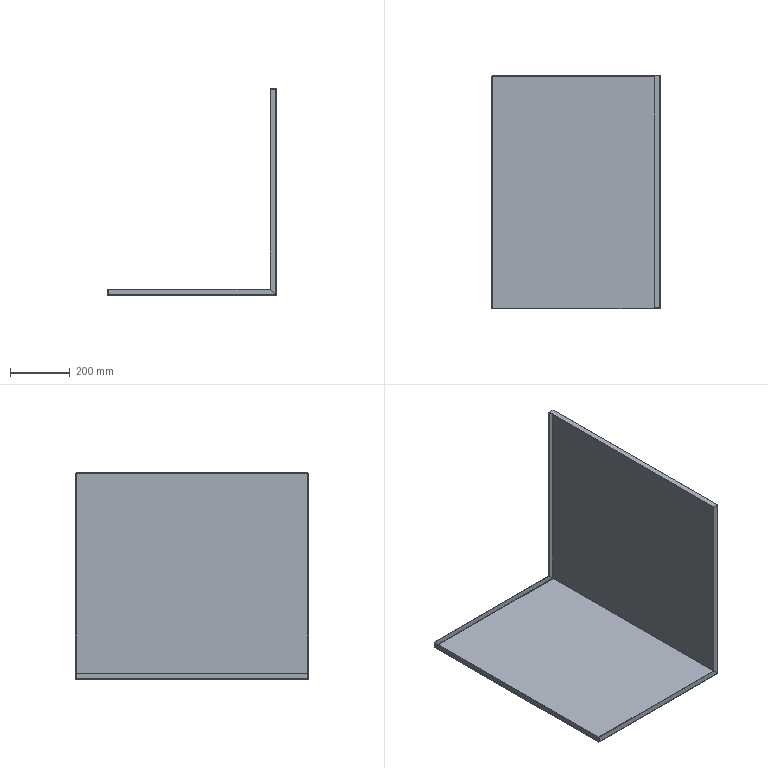Part | STEP file | X77-03023 | 1 solid | 66 faces | box 563 x 778 x 689.5 mm | volume 1566199 mm3 | plane 40 | cylinder 14 | spline 12 | commonest cylinder face diameters 1.473 x7 4.473 x7